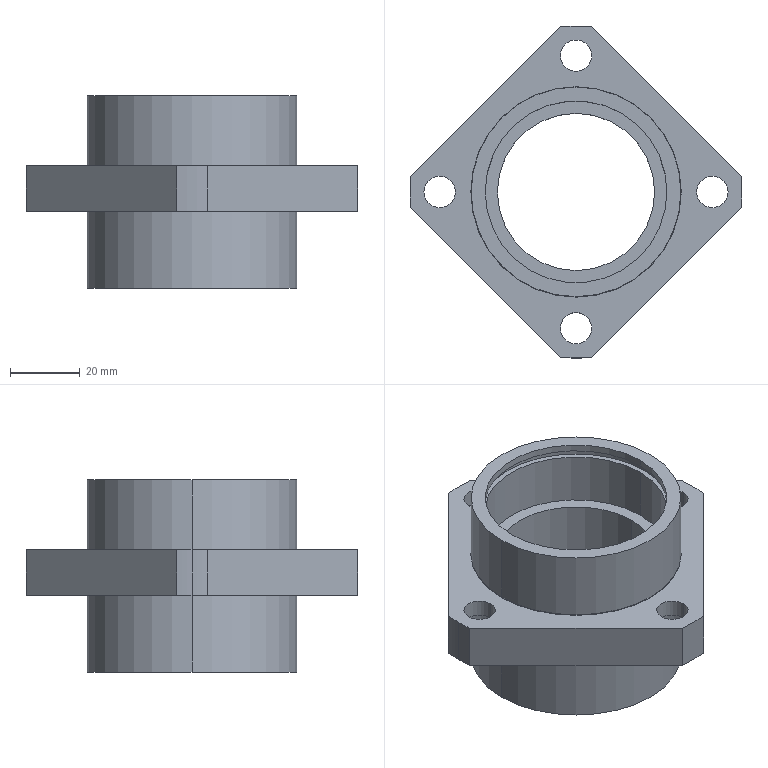Part | STEP file | HI_BFU71-6205ZZ-L55-S20S1^BFU71-6205ZZ-L55-S20_Mechanical tensioner (pay-off) | 1 solid | 59 faces | box 95 x 95 x 55 mm | volume 71824 mm3 | cylinder 39 | plane 18 | torus 2 | commonest cylinder face diameters 9 x8 14 x8 52 x8 95 x5 55 x4 60 x4